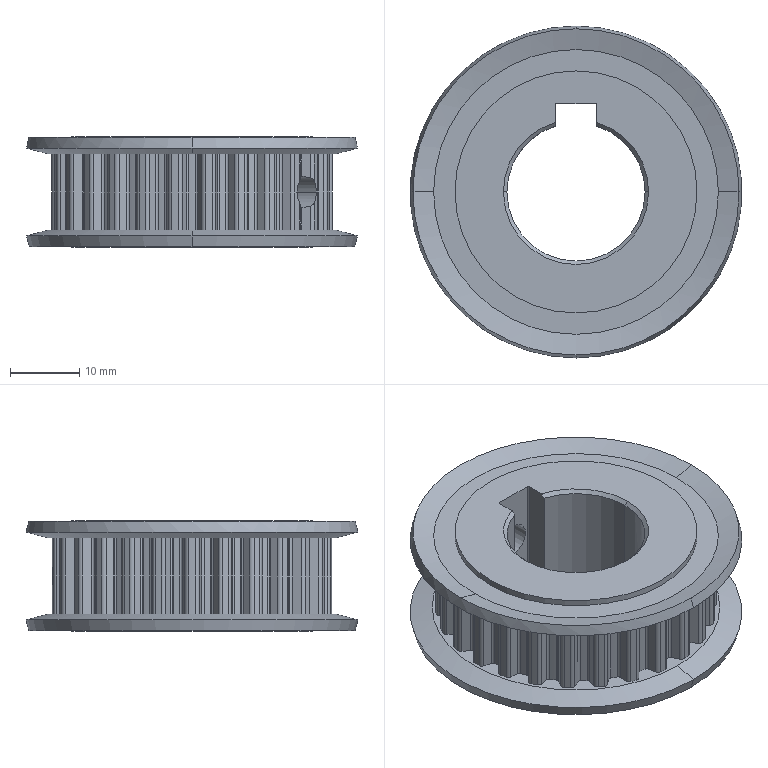Part | STEP file | 1 solid | 284 faces | box 48 x 48 x 16 mm | volume 14884 mm3 | cylinder 201 | plane 65 | cone 18 | commonest cylinder face diameters 1.2 x67 0.8 x66 37 x28 40.6 x27 4.917 x4 35 x4